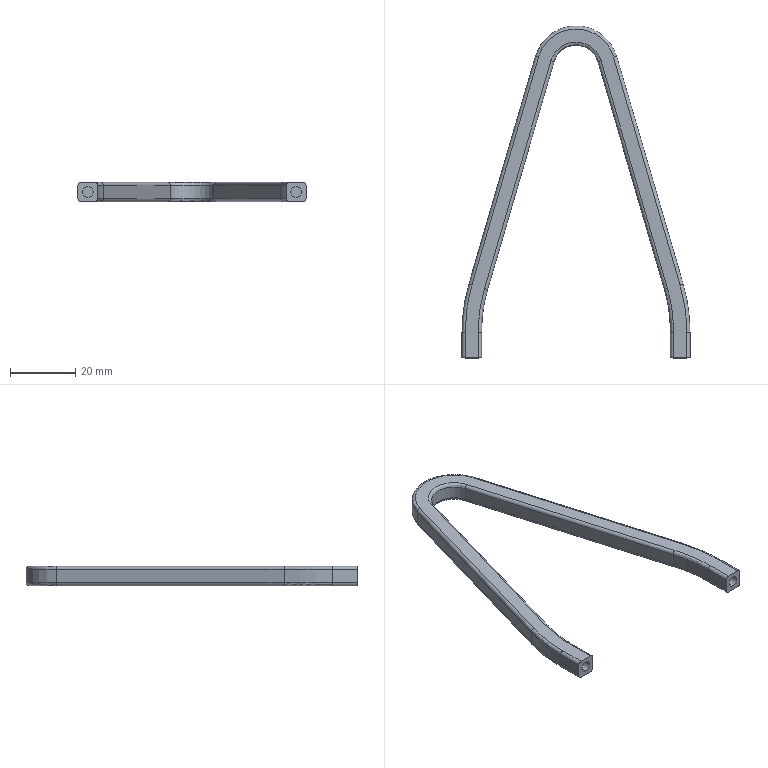Part | STEP file | Stator circlip gauge hook | 1 solid | 52 faces | box 70 x 102 x 6 mm | volume 7420 mm3 | cylinder 26 | plane 14 | spline 12 | commonest cylinder face diameters 2 x16 3.3 x4 94 x2 106 x2 14 x1 26 x1